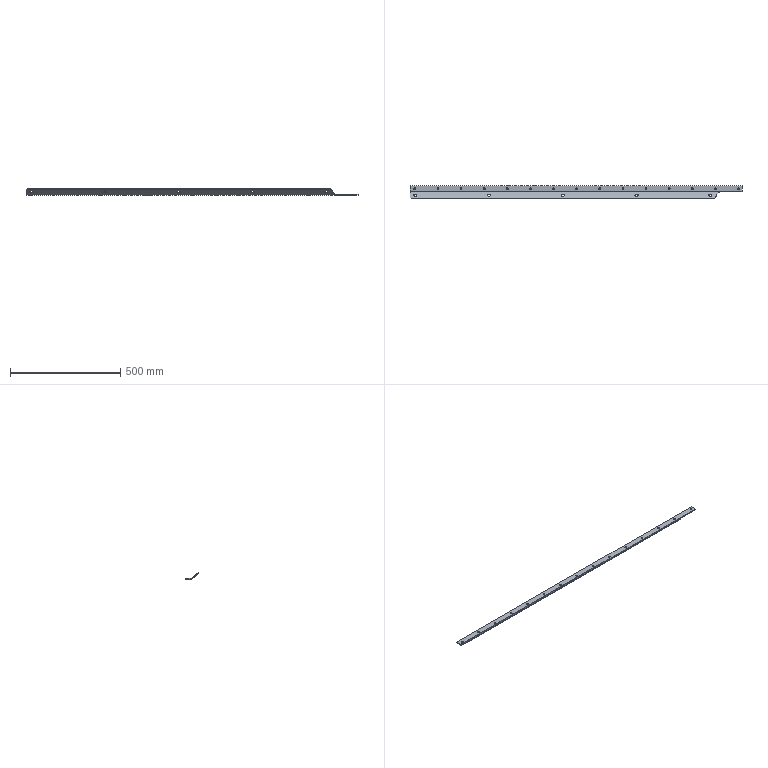Part | SolidWorks | features FlatPattern 1, SM3dBend 1, SMBaseFlange 1, SheetMetal 1 | 1 solid | 58 faces | box 1508 x 59.004 x 28.421 mm | volume 304749 mm3 | cylinder 43 | plane 14 | spline 1 | commonest cylinder face diameters 8 x30 15 x10 10 x1 16.4 x1 20 x1